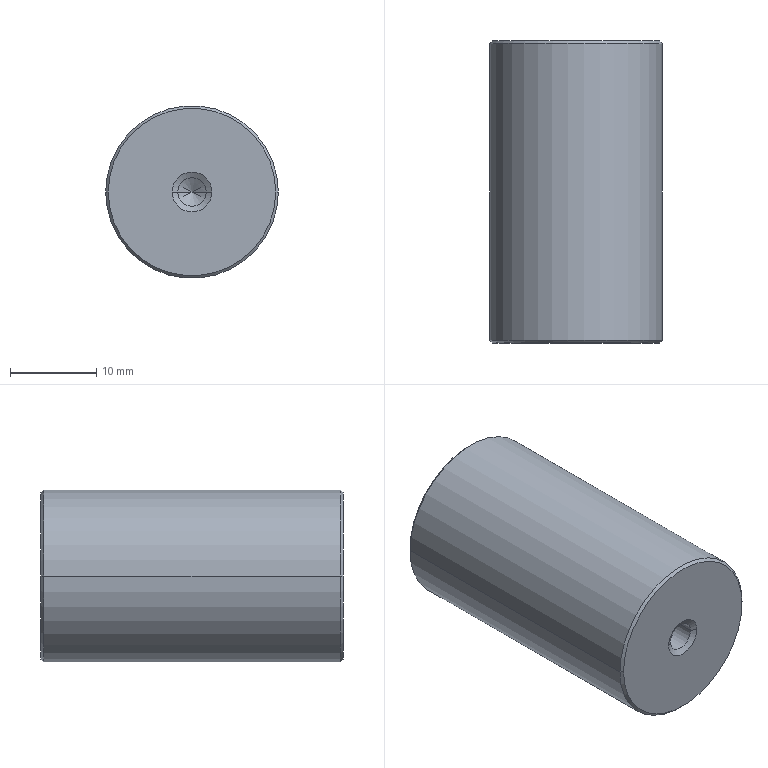Part | NX | 1 solid | 24 faces | box 20 x 35 x 20 mm | volume 10773 mm3 | cone 12 | cylinder 10 | plane 2 | commonest cylinder face diameters 3.3 x8 20 x2
STEP:
#1=CARTESIAN_POINT('',(128.5,-747.8,-755.5));
#2=VERTEX_POINT('',#1);
#3=CARTESIAN_POINT('',(108.5,-747.8,-755.5));
#4=VERTEX_POINT('',#3);
#5=CARTESIAN_POINT('',(118.5,-747.8,-755.5));
#6=DIRECTION('',(0.,1.,0.));
#7=DIRECTION('',(-1.,0.,0.));
#8=AXIS2_PLACEMENT_3D('',#5,#6,#7);
#9=CIRCLE('',#8,10.);
#10=EDGE_CURVE('',#2,#4,#9,.T.);
#11=ORIENTED_EDGE('',*,*,#10,.F.);
#12=CARTESIAN_POINT('',(128.5,-782.2,-755.5));
#13=VERTEX_POINT('',#12);
#14=CARTESIAN_POINT('',(128.5,-782.5,-755.5));
#15=DIRECTION('',(0.,1.,0.));
#16=VECTOR('',#15,1000.);
#17=LINE('',#14,#16);
#18=EDGE_CURVE('',#2,#13,#17,.F.);
#19=ORIENTED_EDGE('',*,*,#18,.T.);
#20=CARTESIAN_POINT('',(108.5,-782.2,-755.5));
#21=VERTEX_POINT('',#20);
#22=CARTESIAN_POINT('',(118.5,-782.2,-755.5));
#23=DIRECTION('',(0.,1.,0.));
#24=DIRECTION('',(-1.,0.,0.));
#25=AXIS2_PLACEMENT_3D('',#22,#23,#24);
#26=CIRCLE('',#25,10.);
#27=EDGE_CURVE('',#13,#21,#26,.T.);
#28=ORIENTED_EDGE('',*,*,#27,.T.);
#29=CARTESIAN_POINT('',(108.5,-782.5,-755.5));
#30=DIRECTION('',(0.,1.,0.));
#31=VECTOR('',#30,1000.);
#32=LINE('',#29,#31);
#33=EDGE_CURVE('',#4,#21,#32,.F.);
#34=ORIENTED_EDGE('',*,*,#33,.F.);
#35=EDGE_LOOP('',(#11,#19,#28,#34));
#36=FACE_BOUND('',#35,.T.);
#37=CARTESIAN_POINT('',(118.5,-782.5,-755.5));
#38=DIRECTION('',(0.,1.,0.));
#39=DIRECTION('',(-1.,0.,0.));
#40=AXIS2_PLACEMENT_3D('',#37,#38,#39);
#41=CYLINDRICAL_SURFACE('',#40,10.);
#42=ADVANCED_FACE('',(#36),#41,.T.);
#43=ORIENTED_EDGE('',*,*,#33,.T.);
#44=CARTESIAN_POINT('',(118.5,-782.2,-755.5));
#45=DIRECTION('',(0.,1.,0.));
#46=DIRECTION('',(-1.,0.,0.));
#47=AXIS2_PLACEMENT_3D('',#44,#45,#46);
#48=CIRCLE('',#47,10.);
#49=EDGE_CURVE('',#21,#13,#48,.T.);
#50=ORIENTED_EDGE('',*,*,#49,.T.);
#51=ORIENTED_EDGE('',*,*,#18,.F.);
#52=CARTESIAN_POINT('',(118.5,-747.8,-755.5));
#53=DIRECTION('',(0.,1.,0.));
#54=DIRECTION('',(-1.,0.,0.));
#55=AXIS2_PLACEMENT_3D('',#52,#53,#54);
#56=CIRCLE('',#55,10.);
#57=EDGE_CURVE('',#4,#2,#56,.T.);
#58=ORIENTED_EDGE('',*,*,#57,.F.);
#59=EDGE_LOOP('',(#43,#50,#51,#58));
#60=FACE_BOUND('',#59,.T.);
#61=CARTESIAN_POINT('',(118.5,-782.5,-755.5));
#62=DIRECTION('',(0.,1.,0.));
#63=DIRECTION('',(-1.,0.,0.));
#64=AXIS2_PLACEMENT_3D('',#61,#62,#63);
#65=CYLINDRICAL_SURFACE('',#64,10.);
#66=ADVANCED_FACE('',(#60),#65,.T.);
#67=CARTESIAN_POINT('',(128.2,-747.5,-755.5));
#68=VERTEX_POINT('',#67);
#69=CARTESIAN_POINT('',(108.8,-747.5,-755.5));
#70=VERTEX_POINT('',#69);
#71=CARTESIAN_POINT('',(118.5,-747.5,-755.5));
#72=DIRECTION('',(0.,1.,0.));
#73=DIRECTION('',(-1.,0.,0.));
#74=AXIS2_PLACEMENT_3D('',#71,#72,#73);
#75=CIRCLE('',#74,9.7);
#76=EDGE_CURVE('',#68,#70,#75,.T.);
#77=ORIENTED_EDGE('',*,*,#76,.T.);
#78=CARTESIAN_POINT('',(118.5,-747.5,-755.5));
#79=DIRECTION('',(0.,1.,0.));
#80=DIRECTION('',(-1.,0.,0.));
#81=AXIS2_PLACEMENT_3D('',#78,#79,#80);
#82=CIRCLE('',#81,9.7);
#83=EDGE_CURVE('',#70,#68,#82,.T.);
#84=ORIENTED_EDGE('',*,*,#83,.T.);
#85=EDGE_LOOP('',(#77,#84));
#86=FACE_BOUND('',#85,.T.);
#87=CARTESIAN_POINT('',(120.815,-747.5,-755.5));
#88=VERTEX_POINT('',#87);
#89=CARTESIAN_POINT('',(116.185,-747.5,-755.5));
#90=VERTEX_POINT('',#89);
#91=CARTESIAN_POINT('',(118.5,-747.5,-755.5));
#92=DIRECTION('',(0.,1.,0.));
#93=DIRECTION('',(-1.,0.,0.));
#94=AXIS2_PLACEMENT_3D('',#91,#92,#93);
#95=CIRCLE('',#94,2.315);
#96=EDGE_CURVE('',#88,#90,#95,.T.);
#97=ORIENTED_EDGE('',*,*,#96,.F.);
#98=CARTESIAN_POINT('',(118.5,-747.5,-755.5));
#99=DIRECTION('',(0.,1.,0.));
#100=DIRECTION('',(-1.,0.,0.));
#101=AXIS2_PLACEMENT_3D('',#98,#99,#100);
#102=CIRCLE('',#101,2.315);
#103=EDGE_CURVE('',#90,#88,#102,.T.);
#104=ORIENTED_EDGE('',*,*,#103,.F.);
#105=EDGE_LOOP('',(#97,#104));
#106=FACE_BOUND('',#105,.T.);
#107=CARTESIAN_POINT('',(692.506,-747.5,-726.749));
#108=DIRECTION('',(0.,1.,0.));
#109=DIRECTION('',(1.,0.,0.));
#110=AXIS2_PLACEMENT_3D('',#107,#108,#109);
#111=PLANE('',#110);
#112=ADVANCED_FACE('',(#86,#106),#111,.T.);
#113=CARTESIAN_POINT('',(120.15,-747.884,-755.5));
#114=VERTEX_POINT('',#113);
#115=CARTESIAN_POINT('',(116.85,-747.884,-755.5));
#116=VERTEX_POINT('',#115);
#117=CARTESIAN_POINT('',(118.5,-747.884,-755.5));
#118=DIRECTION('',(0.,1.,0.));
#119=DIRECTION('',(-1.,0.,0.));
#120=AXIS2_PLACEMENT_3D('',#117,#118,#119);
#121=CIRCLE('',#120,1.65);
#122=EDGE_CURVE('',#114,#116,#121,.T.);
#123=ORIENTED_EDGE('',*,*,#122,.T.);
#124=CARTESIAN_POINT('',(116.85,-755.5,-755.5));
#125=VERTEX_POINT('',#124);
#126=CARTESIAN_POINT('',(116.85,-747.5,-755.5));
#127=DIRECTION('',(0.,1.,0.));
#128=VECTOR('',#127,1000.);
#129=LINE('',#126,#128);
#130=EDGE_CURVE('',#116,#125,#129,.F.);
#131=ORIENTED_EDGE('',*,*,#130,.T.);
#132=CARTESIAN_POINT('',(120.15,-755.5,-755.5));
#133=VERTEX_POINT('',#132);
#134=CARTESIAN_POINT('',(118.5,-755.5,-755.5));
#135=DIRECTION('',(0.,1.,0.));
#136=DIRECTION('',(-1.,0.,0.));
#137=AXIS2_PLACEMENT_3D('',#134,#135,#136);
#138=CIRCLE('',#137,1.65);
#139=EDGE_CURVE('',#133,#125,#138,.T.);
#140=ORIENTED_EDGE('',*,*,#139,.F.);
#141=CARTESIAN_POINT('',(120.15,-747.5,-755.5));
#142=DIRECTION('',(0.,1.,0.));
#143=VECTOR('',#142,1000.);
#144=LINE('',#141,#143);
#145=EDGE_CURVE('',#114,#133,#144,.F.);
#146=ORIENTED_EDGE('',*,*,#145,.F.);
#147=EDGE_LOOP('',(#123,#131,#140,#146));
#148=FACE_BOUND('',#147,.T.);
#149=CARTESIAN_POINT('',(118.5,-747.5,-755.5));
#150=DIRECTION('',(0.,1.,0.));
#151=DIRECTION('',(-1.,0.,0.));
#152=AXIS2_PLACEMENT_3D('',#149,#150,#151);
#153=CYLINDRICAL_SURFACE('',#152,1.65);
#154=ADVANCED_FACE('',(#148),#153,.F.);
#155=ORIENTED_EDGE('',*,*,#139,.T.);
#156=CARTESIAN_POINT('',(116.85,-759.7,-755.5));
#157=VERTEX_POINT('',#156);
#158=CARTESIAN_POINT('',(116.85,-747.5,-755.5));
#159=DIRECTION('',(0.,1.,0.));
#160=VECTOR('',#159,1000.);
#161=LINE('',#158,#160);
#162=EDGE_CURVE('',#125,#157,#161,.F.);
#163=ORIENTED_EDGE('',*,*,#162,.T.);
#164=CARTESIAN_POINT('',(120.15,-759.7,-755.5));
#165=VERTEX_POINT('',#164);
#166=CARTESIAN_POINT('',(118.5,-759.7,-755.5));
#167=DIRECTION('',(0.,1.,0.));
#168=DIRECTION('',(-1.,0.,0.));
#169=AXIS2_PLACEMENT_3D('',#166,#167,#168);
#170=CIRCLE('',#169,1.65);
#171=EDGE_CURVE('',#165,#157,#170,.T.);
#172=ORIENTED_EDGE('',*,*,#171,.F.);
#173=CARTESIAN_POINT('',(120.15,-747.5,-755.5));
#174=DIRECTION('',(0.,1.,0.));
#175=VECTOR('',#174,1000.);
#176=LINE('',#173,#175);
#177=EDGE_CURVE('',#133,#165,#176,.F.);
#178=ORIENTED_EDGE('',*,*,#177,.F.);
#179=EDGE_LOOP('',(#155,#163,#172,#178));
#180=FACE_BOUND('',#179,.T.);
#181=CARTESIAN_POINT('',(118.5,-747.5,-755.5));
#182=DIRECTION('',(0.,1.,0.));
#183=DIRECTION('',(-1.,0.,0.));
#184=AXIS2_PLACEMENT_3D('',#181,#182,#183);
#185=CYLINDRICAL_SURFACE('',#184,1.65);
#186=ADVANCED_FACE('',(#180),#185,.F.);
#187=ORIENTED_EDGE('',*,*,#171,.T.);
#188=CARTESIAN_POINT('',(118.5,-760.691,-755.5));
#189=VERTEX_POINT('',#188);
#190=CARTESIAN_POINT('',(116.85,-759.7,-755.5));
#191=DIRECTION('',(-0.8572,0.515,0.));
#192=VECTOR('',#191,1000.);
#193=LINE('',#190,#192);
#194=EDGE_CURVE('',#189,#157,#193,.T.);
#195=ORIENTED_EDGE('',*,*,#194,.F.);
#196=CARTESIAN_POINT('',(120.15,-759.7,-755.5));
#197=DIRECTION('',(0.8572,0.515,0.));
#198=VECTOR('',#197,1000.);
#199=LINE('',#196,#198);
#200=EDGE_CURVE('',#189,#165,#199,.T.);
#201=ORIENTED_EDGE('',*,*,#200,.T.);
#202=EDGE_LOOP('',(#187,#195,#201));
#203=FACE_BOUND('',#202,.T.);
#204=CARTESIAN_POINT('',(118.5,-759.7,-755.5));
#205=DIRECTION('',(0.,1.,0.));
#206=DIRECTION('',(-1.,0.,0.));
#207=AXIS2_PLACEMENT_3D('',#204,#205,#206);
#208=CONICAL_SURFACE('',#207,1.65,1.03);
#209=ADVANCED_FACE('',(#203),#208,.F.);
#210=ORIENTED_EDGE('',*,*,#122,.F.);
#211=CARTESIAN_POINT('',(120.15,-747.884,-755.5));
#212=DIRECTION('',(0.866,0.5,0.));
#213=VECTOR('',#212,1000.);
#214=LINE('',#211,#213);
#215=EDGE_CURVE('',#88,#114,#214,.F.);
#216=ORIENTED_EDGE('',*,*,#215,.F.);
#217=ORIENTED_EDGE('',*,*,#96,.T.);
#218=CARTESIAN_POINT('',(116.85,-747.884,-755.5));
#219=DIRECTION('',(-0.866,0.5,0.));
#220=VECTOR('',#219,1000.);
#221=LINE('',#218,#220);
#222=EDGE_CURVE('',#90,#116,#221,.F.);
#223=ORIENTED_EDGE('',*,*,#222,.T.);
#224=EDGE_LOOP('',(#210,#216,#217,#223));
#225=FACE_BOUND('',#224,.T.);
#226=CARTESIAN_POINT('',(118.5,-747.884,-755.5));
#227=DIRECTION('',(0.,1.,0.));
#228=DIRECTION('',(-1.,0.,0.));
#229=AXIS2_PLACEMENT_3D('',#226,#227,#228);
#230=CONICAL_SURFACE('',#229,1.65,1.047);
#231=ADVANCED_FACE('',(#225),#230,.F.);
#232=CARTESIAN_POINT('',(116.85,-782.116,-755.5));
#233=VERTEX_POINT('',#232);
#234=CARTESIAN_POINT('',(120.15,-782.116,-755.5));
#235=VERTEX_POINT('',#234);
#236=CARTESIAN_POINT('',(118.5,-782.116,-755.5));
#237=DIRECTION('',(0.,-1.,0.));
#238=DIRECTION('',(1.,0.,0.));
#239=AXIS2_PLACEMENT_3D('',#236,#237,#238);
#240=CIRCLE('',#239,1.65);
#241=EDGE_CURVE('',#233,#235,#240,.T.);
#242=ORIENTED_EDGE('',*,*,#241,.T.);
#243=CARTESIAN_POINT('',(120.15,-774.5,-755.5));
#244=VERTEX_POINT('',#243);
#245=CARTESIAN_POINT('',(120.15,-782.5,-755.5));
#246=DIRECTION('',(0.,-1.,0.));
#247=VECTOR('',#246,1000.);
#248=LINE('',#245,#247);
#249=EDGE_CURVE('',#244,#235,#248,.T.);
#250=ORIENTED_EDGE('',*,*,#249,.F.);
#251=CARTESIAN_POINT('',(116.85,-774.5,-755.5));
#252=VERTEX_POINT('',#251);
#253=CARTESIAN_POINT('',(118.5,-774.5,-755.5));
#254=DIRECTION('',(0.,-1.,0.));
#255=DIRECTION('',(1.,0.,0.));
#256=AXIS2_PLACEMENT_3D('',#253,#254,#255);
#257=CIRCLE('',#256,1.65);
#258=EDGE_CURVE('',#252,#244,#257,.T.);
#259=ORIENTED_EDGE('',*,*,#258,.F.);
#260=CARTESIAN_POINT('',(116.85,-782.5,-755.5));
#261=DIRECTION('',(0.,-1.,0.));
#262=VECTOR('',#261,1000.);
#263=LINE('',#260,#262);
#264=EDGE_CURVE('',#252,#233,#263,.T.);
#265=ORIENTED_EDGE('',*,*,#264,.T.);
#266=EDGE_LOOP('',(#242,#250,#259,#265));
#267=FACE_BOUND('',#266,.T.);
#268=CARTESIAN_POINT('',(118.5,-782.5,-755.5));
#269=DIRECTION('',(0.,-1.,0.));
#270=DIRECTION('',(1.,0.,0.));
#271=AXIS2_PLACEMENT_3D('',#268,#269,#270);
#272=CYLINDRICAL_SURFACE('',#271,1.65);
#273=ADVANCED_FACE('',(#267),#272,.F.);
#274=ORIENTED_EDGE('',*,*,#258,.T.);
#275=CARTESIAN_POINT('',(120.15,-770.3,-755.5));
#276=VERTEX_POINT('',#275);
#277=CARTESIAN_POINT('',(120.15,-782.5,-755.5));
#278=DIRECTION('',(0.,-1.,0.));
#279=VECTOR('',#278,1000.);
#280=LINE('',#277,#279);
#281=EDGE_CURVE('',#276,#244,#280,.T.);
#282=ORIENTED_EDGE('',*,*,#281,.F.);
#283=CARTESIAN_POINT('',(116.85,-770.3,-755.5));
#284=VERTEX_POINT('',#283);
#285=CARTESIAN_POINT('',(118.5,-770.3,-755.5));
#286=DIRECTION('',(0.,-1.,0.));
#287=DIRECTION('',(1.,0.,0.));
#288=AXIS2_PLACEMENT_3D('',#285,#286,#287);
#289=CIRCLE('',#288,1.65);
#290=EDGE_CURVE('',#284,#276,#289,.T.);
#291=ORIENTED_EDGE('',*,*,#290,.F.);
#292=CARTESIAN_POINT('',(116.85,-782.5,-755.5));
#293=DIRECTION('',(0.,-1.,0.));
#294=VECTOR('',#293,1000.);
#295=LINE('',#292,#294);
#296=EDGE_CURVE('',#284,#252,#295,.T.);
#297=ORIENTED_EDGE('',*,*,#296,.T.);
#298=EDGE_LOOP('',(#274,#282,#291,#297));
#299=FACE_BOUND('',#298,.T.);
#300=CARTESIAN_POINT('',(118.5,-782.5,-755.5));
#301=DIRECTION('',(0.,-1.,0.));
#302=DIRECTION('',(1.,0.,0.));
#303=AXIS2_PLACEMENT_3D('',#300,#301,#302);
#304=CYLINDRICAL_SURFACE('',#303,1.65);
#305=ADVANCED_FACE('',(#299),#304,.F.);
#306=ORIENTED_EDGE('',*,*,#290,.T.);
#307=CARTESIAN_POINT('',(118.5,-769.309,-755.5));
#308=VERTEX_POINT('',#307);
#309=CARTESIAN_POINT('',(120.15,-770.3,-755.5));
#310=DIRECTION('',(0.8572,-0.515,0.));
#311=VECTOR('',#310,1000.);
#312=LINE('',#309,#311);
#313=EDGE_CURVE('',#276,#308,#312,.F.);
#314=ORIENTED_EDGE('',*,*,#313,.T.);
#315=CARTESIAN_POINT('',(116.85,-770.3,-755.5));
#316=DIRECTION('',(-0.8572,-0.515,0.));
#317=VECTOR('',#316,1000.);
#318=LINE('',#315,#317);
#319=EDGE_CURVE('',#284,#308,#318,.F.);
#320=ORIENTED_EDGE('',*,*,#319,.F.);
#321=EDGE_LOOP('',(#306,#314,#320));
#322=FACE_BOUND('',#321,.T.);
#323=CARTESIAN_POINT('',(118.5,-770.3,-755.5));
#324=DIRECTION('',(0.,-1.,0.));
#325=DIRECTION('',(1.,0.,0.));
#326=AXIS2_PLACEMENT_3D('',#323,#324,#325);
#327=CONICAL_SURFACE('',#326,1.65,1.03);
#328=ADVANCED_FACE('',(#322),#327,.F.);
#329=ORIENTED_EDGE('',*,*,#241,.F.);
#330=CARTESIAN_POINT('',(116.185,-782.5,-755.5));
#331=VERTEX_POINT('',#330);
#332=CARTESIAN_POINT('',(116.85,-782.116,-755.5));
#333=DIRECTION('',(-0.866,-0.5,0.));
#334=VECTOR('',#333,1000.);
#335=LINE('',#332,#334);
#336=EDGE_CURVE('',#233,#331,#335,.T.);
#337=ORIENTED_EDGE('',*,*,#336,.T.);
#338=CARTESIAN_POINT('',(120.815,-782.5,-755.5));
#339=VERTEX_POINT('',#338);
#340=CARTESIAN_POINT('',(118.5,-782.5,-755.5));
#341=DIRECTION('',(0.,-1.,0.));
#342=DIRECTION('',(1.,0.,0.));
#343=AXIS2_PLACEMENT_3D('',#340,#341,#342);
#344=CIRCLE('',#343,2.315);
#345=EDGE_CURVE('',#331,#339,#344,.T.);
#346=ORIENTED_EDGE('',*,*,#345,.T.);
#347=CARTESIAN_POINT('',(120.15,-782.116,-755.5));
#348=DIRECTION('',(0.866,-0.5,0.));
#349=VECTOR('',#348,1000.);
#350=LINE('',#347,#349);
#351=EDGE_CURVE('',#235,#339,#350,.T.);
#352=ORIENTED_EDGE('',*,*,#351,.F.);
#353=EDGE_LOOP('',(#329,#337,#346,#352));
#354=FACE_BOUND('',#353,.T.);
#355=CARTESIAN_POINT('',(118.5,-782.116,-755.5));
#356=DIRECTION('',(0.,-1.,0.));
#357=DIRECTION('',(1.,0.,0.));
#358=AXIS2_PLACEMENT_3D('',#355,#356,#357);
#359=CONICAL_SURFACE('',#358,1.65,1.047);
#360=ADVANCED_FACE('',(#354),#359,.F.);
#361=ORIENTED_EDGE('',*,*,#76,.F.);
#362=CARTESIAN_POINT('',(128.2,-747.5,-755.5));
#363=DIRECTION('',(0.7071,-0.7071,0.));
#364=VECTOR('',#363,1000.);
#365=LINE('',#362,#364);
#366=EDGE_CURVE('',#68,#2,#365,.T.);
#367=ORIENTED_EDGE('',*,*,#366,.T.);
#368=ORIENTED_EDGE('',*,*,#10,.T.);
#369=CARTESIAN_POINT('',(108.8,-747.5,-755.5));
#370=DIRECTION('',(-0.7071,-0.7071,0.));
#371=VECTOR('',#370,1000.);
#372=LINE('',#369,#371);
#373=EDGE_CURVE('',#70,#4,#372,.T.);
#374=ORIENTED_EDGE('',*,*,#373,.F.);
#375=EDGE_LOOP('',(#361,#367,#368,#374));
#376=FACE_BOUND('',#375,.T.);
#377=CARTESIAN_POINT('',(118.5,-747.5,-755.5));
#378=DIRECTION('',(0.,-1.,0.));
#379=DIRECTION('',(1.,0.,0.));
#380=AXIS2_PLACEMENT_3D('',#377,#378,#379);
#381=CONICAL_SURFACE('',#380,9.7,0.7854);
#382=ADVANCED_FACE('',(#376),#381,.T.);
#383=ORIENTED_EDGE('',*,*,#366,.F.);
#384=ORIENTED_EDGE('',*,*,#83,.F.);
#385=ORIENTED_EDGE('',*,*,#373,.T.);
#386=ORIENTED_EDGE('',*,*,#57,.T.);
#387=EDGE_LOOP('',(#383,#384,#385,#386));
#388=FACE_BOUND('',#387,.T.);
#389=CARTESIAN_POINT('',(118.5,-747.5,-755.5));
#390=DIRECTION('',(0.,-1.,0.));
#391=DIRECTION('',(1.,0.,0.));
#392=AXIS2_PLACEMENT_3D('',#389,#390,#391);
#393=CONICAL_SURFACE('',#392,9.7,0.7854);
#394=ADVANCED_FACE('',(#388),#393,.T.);
#395=ORIENTED_EDGE('',*,*,#162,.F.);
#396=CARTESIAN_POINT('',(118.5,-755.5,-755.5));
#397=DIRECTION('',(0.,1.,0.));
#398=DIRECTION('',(-1.,0.,0.));
#399=AXIS2_PLACEMENT_3D('',#396,#397,#398);
#400=CIRCLE('',#399,1.65);
#401=EDGE_CURVE('',#125,#133,#400,.T.);
#402=ORIENTED_EDGE('',*,*,#401,.T.);
#403=ORIENTED_EDGE('',*,*,#177,.T.);
#404=CARTESIAN_POINT('',(118.5,-759.7,-755.5));
#405=DIRECTION('',(0.,1.,0.));
#406=DIRECTION('',(-1.,0.,0.));
#407=AXIS2_PLACEMENT_3D('',#404,#405,#406);
#408=CIRCLE('',#407,1.65);
#409=EDGE_CURVE('',#157,#165,#408,.T.);
#410=ORIENTED_EDGE('',*,*,#409,.F.);
#411=EDGE_LOOP('',(#395,#402,#403,#410));
#412=FACE_BOUND('',#411,.T.);
#413=CARTESIAN_POINT('',(118.5,-747.5,-755.5));
#414=DIRECTION('',(0.,1.,0.));
#415=DIRECTION('',(-1.,0.,0.));
#416=AXIS2_PLACEMENT_3D('',#413,#414,#415);
#417=CYLINDRICAL_SURFACE('',#416,1.65);
#418=ADVANCED_FACE('',(#412),#417,.F.);
#419=ORIENTED_EDGE('',*,*,#319,.T.);
#420=ORIENTED_EDGE('',*,*,#313,.F.);
#421=CARTESIAN_POINT('',(118.5,-770.3,-755.5));
#422=DIRECTION('',(0.,-1.,0.));
#423=DIRECTION('',(1.,0.,0.));
#424=AXIS2_PLACEMENT_3D('',#421,#422,#423);
#425=CIRCLE('',#424,1.65);
#426=EDGE_CURVE('',#276,#284,#425,.T.);
#427=ORIENTED_EDGE('',*,*,#426,.T.);
#428=EDGE_LOOP('',(#419,#420,#427));
#429=FACE_BOUND('',#428,.T.);
#430=CARTESIAN_POINT('',(118.5,-770.3,-755.5));
#431=DIRECTION('',(0.,-1.,0.));
#432=DIRECTION('',(1.,0.,0.));
#433=AXIS2_PLACEMENT_3D('',#430,#431,#432);
#434=CONICAL_SURFACE('',#433,1.65,1.03);
#435=ADVANCED_FACE('',(#429),#434,.F.);
#436=ORIENTED_EDGE('',*,*,#351,.T.);
#437=CARTESIAN_POINT('',(118.5,-782.5,-755.5));
#438=DIRECTION('',(0.,-1.,0.));
#439=DIRECTION('',(1.,0.,0.));
#440=AXIS2_PLACEMENT_3D('',#437,#438,#439);
#441=CIRCLE('',#440,2.315);
#442=EDGE_CURVE('',#339,#331,#441,.T.);
#443=ORIENTED_EDGE('',*,*,#442,.T.);
#444=ORIENTED_EDGE('',*,*,#336,.F.);
#445=CARTESIAN_POINT('',(118.5,-782.116,-755.5));
#446=DIRECTION('',(0.,-1.,0.));
#447=DIRECTION('',(1.,0.,0.));
#448=AXIS2_PLACEMENT_3D('',#445,#446,#447);
#449=CIRCLE('',#448,1.65);
#450=EDGE_CURVE('',#235,#233,#449,.T.);
#451=ORIENTED_EDGE('',*,*,#450,.F.);
#452=EDGE_LOOP('',(#436,#443,#444,#451));
#453=FACE_BOUND('',#452,.T.);
#454=CARTESIAN_POINT('',(118.5,-782.116,-755.5));
#455=DIRECTION('',(0.,-1.,0.));
#456=DIRECTION('',(1.,0.,0.));
#457=AXIS2_PLACEMENT_3D('',#454,#455,#456);
#458=CONICAL_SURFACE('',#457,1.65,1.047);
#459=ADVANCED_FACE('',(#453),#458,.F.);
#460=ORIENTED_EDGE('',*,*,#200,.F.);
#461=ORIENTED_EDGE('',*,*,#194,.T.);
#462=ORIENTED_EDGE('',*,*,#409,.T.);
#463=EDGE_LOOP('',(#460,#461,#462));
#464=FACE_BOUND('',#463,.T.);
#465=CARTESIAN_POINT('',(118.5,-759.7,-755.5));
#466=DIRECTION('',(0.,1.,0.));
#467=DIRECTION('',(-1.,0.,0.));
#468=AXIS2_PLACEMENT_3D('',#465,#466,#467);
#469=CONICAL_SURFACE('',#468,1.65,1.03);
#470=ADVANCED_FACE('',(#464),#469,.F.);
#471=ORIENTED_EDGE('',*,*,#222,.F.);
#472=ORIENTED_EDGE('',*,*,#103,.T.);
#473=ORIENTED_EDGE('',*,*,#215,.T.);
#474=CARTESIAN_POINT('',(118.5,-747.884,-755.5));
#475=DIRECTION('',(0.,1.,0.));
#476=DIRECTION('',(-1.,0.,0.));
#477=AXIS2_PLACEMENT_3D('',#474,#475,#476);
#478=CIRCLE('',#477,1.65);
#479=EDGE_CURVE('',#116,#114,#478,.T.);
#480=ORIENTED_EDGE('',*,*,#479,.F.);
#481=EDGE_LOOP('',(#471,#472,#473,#480));
#482=FACE_BOUND('',#481,.T.);
#483=CARTESIAN_POINT('',(118.5,-747.884,-755.5));
#484=DIRECTION('',(0.,1.,0.));
#485=DIRECTION('',(-1.,0.,0.));
#486=AXIS2_PLACEMENT_3D('',#483,#484,#485);
#487=CONICAL_SURFACE('',#486,1.65,1.047);
#488=ADVANCED_FACE('',(#482),#487,.F.);
#489=ORIENTED_EDGE('',*,*,#249,.T.);
#490=ORIENTED_EDGE('',*,*,#450,.T.);
#491=ORIENTED_EDGE('',*,*,#264,.F.);
#492=CARTESIAN_POINT('',(118.5,-774.5,-755.5));
#493=DIRECTION('',(0.,-1.,0.));
#494=DIRECTION('',(1.,0.,0.));
#495=AXIS2_PLACEMENT_3D('',#492,#493,#494);
#496=CIRCLE('',#495,1.65);
#497=EDGE_CURVE('',#244,#252,#496,.T.);
#498=ORIENTED_EDGE('',*,*,#497,.F.);
#499=EDGE_LOOP('',(#489,#490,#491,#498));
#500=FACE_BOUND('',#499,.T.);
#501=CARTESIAN_POINT('',(118.5,-782.5,-755.5));
#502=DIRECTION('',(0.,-1.,0.));
#503=DIRECTION('',(1.,0.,0.));
#504=AXIS2_PLACEMENT_3D('',#501,#502,#503);
#505=CYLINDRICAL_SURFACE('',#504,1.65);
#506=ADVANCED_FACE('',(#500),#505,.F.);
#507=ORIENTED_EDGE('',*,*,#130,.F.);
#508=ORIENTED_EDGE('',*,*,#479,.T.);
#509=ORIENTED_EDGE('',*,*,#145,.T.);
#510=ORIENTED_EDGE('',*,*,#401,.F.);
#511=EDGE_LOOP('',(#507,#508,#509,#510));
#512=FACE_BOUND('',#511,.T.);
#513=CARTESIAN_POINT('',(118.5,-747.5,-755.5));
#514=DIRECTION('',(0.,1.,0.));
#515=DIRECTION('',(-1.,0.,0.));
#516=AXIS2_PLACEMENT_3D('',#513,#514,#515);
#517=CYLINDRICAL_SURFACE('',#516,1.65);
#518=ADVANCED_FACE('',(#512),#517,.F.);
#519=ORIENTED_EDGE('',*,*,#281,.T.);
#520=ORIENTED_EDGE('',*,*,#497,.T.);
#521=ORIENTED_EDGE('',*,*,#296,.F.);
#522=ORIENTED_EDGE('',*,*,#426,.F.);
#523=EDGE_LOOP('',(#519,#520,#521,#522));
#524=FACE_BOUND('',#523,.T.);
#525=CARTESIAN_POINT('',(118.5,-782.5,-755.5));
#526=DIRECTION('',(0.,-1.,0.));
#527=DIRECTION('',(1.,0.,0.));
#528=AXIS2_PLACEMENT_3D('',#525,#526,#527);
#529=CYLINDRICAL_SURFACE('',#528,1.65);
#530=ADVANCED_FACE('',(#524),#529,.F.);
#531=CARTESIAN_POINT('',(128.2,-782.5,-755.5));
#532=VERTEX_POINT('',#531);
#533=CARTESIAN_POINT('',(108.8,-782.5,-755.5));
#534=VERTEX_POINT('',#533);
#535=CARTESIAN_POINT('',(118.5,-782.5,-755.5));
#536=DIRECTION('',(0.,1.,0.));
#537=DIRECTION('',(-1.,0.,0.));
#538=AXIS2_PLACEMENT_3D('',#535,#536,#537);
#539=CIRCLE('',#538,9.7);
#540=EDGE_CURVE('',#532,#534,#539,.T.);
#541=ORIENTED_EDGE('',*,*,#540,.F.);
#542=CARTESIAN_POINT('',(118.5,-782.5,-755.5));
#543=DIRECTION('',(0.,1.,0.));
#544=DIRECTION('',(-1.,0.,0.));
#545=AXIS2_PLACEMENT_3D('',#542,#543,#544);
#546=CIRCLE('',#545,9.7);
#547=EDGE_CURVE('',#534,#532,#546,.T.);
#548=ORIENTED_EDGE('',*,*,#547,.F.);
#549=EDGE_LOOP('',(#541,#548));
#550=FACE_BOUND('',#549,.T.);
#551=ORIENTED_EDGE('',*,*,#345,.F.);
#552=ORIENTED_EDGE('',*,*,#442,.F.);
#553=EDGE_LOOP('',(#551,#552));
#554=FACE_BOUND('',#553,.T.);
#555=CARTESIAN_POINT('',(692.506,-782.5,-726.749));
#556=DIRECTION('',(0.,1.,0.));
#557=DIRECTION('',(1.,0.,0.));
#558=AXIS2_PLACEMENT_3D('',#555,#556,#557);
#559=PLANE('',#558);
#560=ADVANCED_FACE('',(#550,#554),#559,.F.);
#561=ORIENTED_EDGE('',*,*,#540,.T.);
#562=CARTESIAN_POINT('',(108.8,-782.5,-755.5));
#563=DIRECTION('',(-0.7071,0.7071,0.));
#564=VECTOR('',#563,1000.);
#565=LINE('',#562,#564);
#566=EDGE_CURVE('',#21,#534,#565,.F.);
#567=ORIENTED_EDGE('',*,*,#566,.F.);
#568=ORIENTED_EDGE('',*,*,#27,.F.);
#569=CARTESIAN_POINT('',(128.2,-782.5,-755.5));
#570=DIRECTION('',(0.7071,0.7071,0.));
#571=VECTOR('',#570,1000.);
#572=LINE('',#569,#571);
#573=EDGE_CURVE('',#13,#532,#572,.F.);
#574=ORIENTED_EDGE('',*,*,#573,.T.);
#575=EDGE_LOOP('',(#561,#567,#568,#574));
#576=FACE_BOUND('',#575,.T.);
#577=CARTESIAN_POINT('',(118.5,-782.5,-755.5));
#578=DIRECTION('',(0.,1.,0.));
#579=DIRECTION('',(-1.,0.,0.));
#580=AXIS2_PLACEMENT_3D('',#577,#578,#579);
#581=CONICAL_SURFACE('',#580,9.7,0.7854);
#582=ADVANCED_FACE('',(#576),#581,.T.);
#583=ORIENTED_EDGE('',*,*,#566,.T.);
#584=ORIENTED_EDGE('',*,*,#547,.T.);
#585=ORIENTED_EDGE('',*,*,#573,.F.);
#586=ORIENTED_EDGE('',*,*,#49,.F.);
#587=EDGE_LOOP('',(#583,#584,#585,#586));
#588=FACE_BOUND('',#587,.T.);
#589=CARTESIAN_POINT('',(118.5,-782.5,-755.5));
#590=DIRECTION('',(0.,1.,0.));
#591=DIRECTION('',(-1.,0.,0.));
#592=AXIS2_PLACEMENT_3D('',#589,#590,#591);
#593=CONICAL_SURFACE('',#592,9.7,0.7854);
#594=ADVANCED_FACE('',(#588),#593,.T.);
#595=CLOSED_SHELL('',(#42,#66,#112,#154,#186,#209,#231,#273,#305,#328,#360,#382,#394,#418,#435,#459,#470,#488,#506,#518,#530,#560,#582,#594));
#596=MANIFOLD_SOLID_BREP('',#595);
#597=(LENGTH_UNIT()NAMED_UNIT(*)SI_UNIT(.MILLI.,.METRE.));
#598=UNCERTAINTY_MEASURE_WITH_UNIT(LENGTH_MEASURE(0.00001),#597,'','');
#599=(NAMED_UNIT(*)PLANE_ANGLE_UNIT()SI_UNIT($,.RADIAN.));
#600=(NAMED_UNIT(*)SI_UNIT($,.STERADIAN.)SOLID_ANGLE_UNIT());
#601=(GEOMETRIC_REPRESENTATION_CONTEXT(3)GLOBAL_UNCERTAINTY_ASSIGNED_CONTEXT((#598))GLOBAL_UNIT_ASSIGNED_CONTEXT((#597,#599,#600))REPRESENTATION_CONTEXT('',''));
#602=ADVANCED_BREP_SHAPE_REPRESENTATION('',(#596),#601);